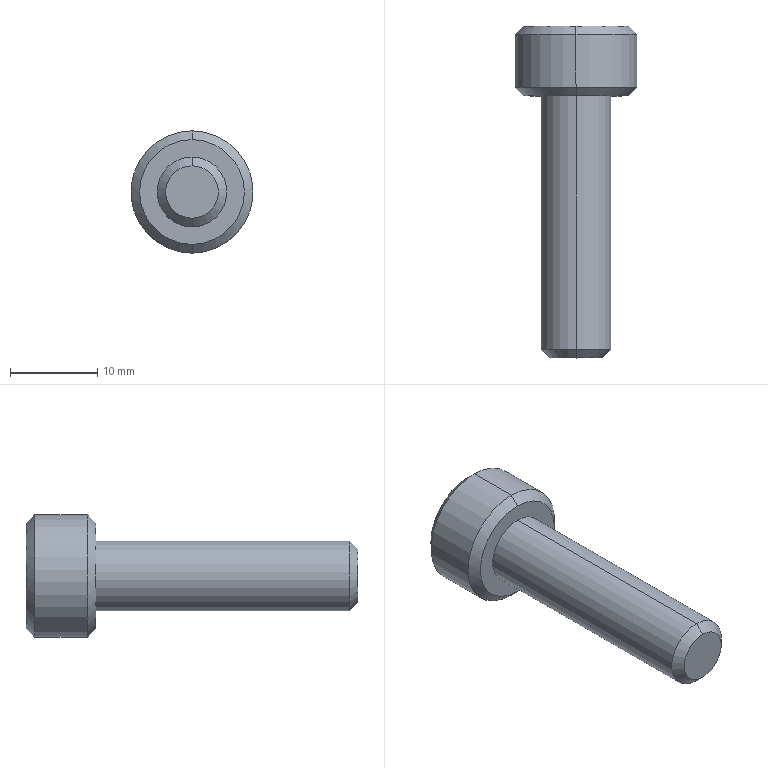Part | STEP file | Vibration plate 3-05_default | 1 solid | 20 faces | box 14 x 38 x 14 mm | volume 2499 mm3 | plane 10 | cone 6 | cylinder 4 | commonest cylinder face diameters 8 x2 14 x2
STEP:
#1=CARTESIAN_POINT('',(0.,0.,0.));
#2=DIRECTION('',(0.,0.,1.));
#3=DIRECTION('',(1.,0.,0.));
#4=AXIS2_PLACEMENT_3D('',#1,#2,#3);
#5=CARTESIAN_POINT('',(0.,1.,4.));
#6=VERTEX_POINT('',#5);
#7=CARTESIAN_POINT('',(0.,1.,-4.));
#8=VERTEX_POINT('',#7);
#9=CARTESIAN_POINT('',(0.,1.,0.));
#10=DIRECTION('',(0.,1.,0.));
#11=DIRECTION('',(0.,0.,1.));
#12=AXIS2_PLACEMENT_3D('',#9,#10,#11);
#13=CIRCLE('',#12,4.);
#14=CARTESIAN_POINT('',(0.,0.,0.));
#15=DIRECTION('',(0.,1.,0.));
#16=DIRECTION('',(0.,0.,1.));
#17=AXIS2_PLACEMENT_3D('',#14,#15,#16);
#18=CYLINDRICAL_SURFACE('',#17,4.);
#19=CARTESIAN_POINT('',(0.,1.));
#20=DIRECTION('',(1.,0.));
#21=VECTOR('',#20,1.);
#22=LINE('',#19,#21);
#23=(GEOMETRIC_REPRESENTATION_CONTEXT(2)PARAMETRIC_REPRESENTATION_CONTEXT()REPRESENTATION_CONTEXT('',''));
#24=DEFINITIONAL_REPRESENTATION('',(#22),#23);
#25=PCURVE('',#18,#24);
#26=CARTESIAN_POINT('',(0.,1.,0.));
#27=DIRECTION('',(0.,1.,0.));
#28=DIRECTION('',(0.,0.,1.));
#29=AXIS2_PLACEMENT_3D('',#26,#27,#28);
#30=CONICAL_SURFACE('',#29,4.,0.7854);
#31=CARTESIAN_POINT('',(0.,0.000008212));
#32=DIRECTION('',(1.,0.));
#33=VECTOR('',#32,1.);
#34=LINE('',#31,#33);
#35=(GEOMETRIC_REPRESENTATION_CONTEXT(2)PARAMETRIC_REPRESENTATION_CONTEXT()REPRESENTATION_CONTEXT('',''));
#36=DEFINITIONAL_REPRESENTATION('',(#34),#35);
#37=PCURVE('',#30,#36);
#38=SURFACE_CURVE('',#13,(#25,#37),.PCURVE_S1.);
#39=EDGE_CURVE('',#6,#8,#38,.T.);
#40=ORIENTED_EDGE('',*,*,#39,.T.);
#41=CARTESIAN_POINT('',(0.,30.,-4.));
#42=VERTEX_POINT('',#41);
#43=CARTESIAN_POINT('',(0.,0.,-4.));
#44=DIRECTION('',(0.,1.,0.));
#45=VECTOR('',#44,1.);
#46=LINE('',#43,#45);
#47=CARTESIAN_POINT('',(3.142,0.));
#48=DIRECTION('',(0.,1.));
#49=VECTOR('',#48,1.);
#50=LINE('',#47,#49);
#51=(GEOMETRIC_REPRESENTATION_CONTEXT(2)PARAMETRIC_REPRESENTATION_CONTEXT()REPRESENTATION_CONTEXT('',''));
#52=DEFINITIONAL_REPRESENTATION('',(#50),#51);
#53=PCURVE('',#18,#52);
#54=CARTESIAN_POINT('',(0.,0.,0.));
#55=DIRECTION('',(0.,1.,0.));
#56=DIRECTION('',(0.,0.,1.));
#57=AXIS2_PLACEMENT_3D('',#54,#55,#56);
#58=CYLINDRICAL_SURFACE('',#57,4.);
#59=CARTESIAN_POINT('',(3.142,0.));
#60=DIRECTION('',(0.,1.));
#61=VECTOR('',#60,1.);
#62=LINE('',#59,#61);
#63=(GEOMETRIC_REPRESENTATION_CONTEXT(2)PARAMETRIC_REPRESENTATION_CONTEXT()REPRESENTATION_CONTEXT('',''));
#64=DEFINITIONAL_REPRESENTATION('',(#62),#63);
#65=PCURVE('',#58,#64);
#66=SURFACE_CURVE('',#46,(#53,#65),.PCURVE_S1.);
#67=EDGE_CURVE('',#8,#42,#66,.T.);
#68=ORIENTED_EDGE('',*,*,#67,.T.);
#69=CARTESIAN_POINT('',(0.,30.,4.));
#70=VERTEX_POINT('',#69);
#71=CARTESIAN_POINT('',(0.,30.,0.));
#72=DIRECTION('',(0.,-1.,0.));
#73=DIRECTION('',(0.,0.,1.));
#74=AXIS2_PLACEMENT_3D('',#71,#72,#73);
#75=CIRCLE('',#74,4.);
#76=CARTESIAN_POINT('',(6.283,30.));
#77=DIRECTION('',(-1.,0.));
#78=VECTOR('',#77,1.);
#79=LINE('',#76,#78);
#80=(GEOMETRIC_REPRESENTATION_CONTEXT(2)PARAMETRIC_REPRESENTATION_CONTEXT()REPRESENTATION_CONTEXT('',''));
#81=DEFINITIONAL_REPRESENTATION('',(#79),#80);
#82=PCURVE('',#18,#81);
#83=CARTESIAN_POINT('',(0.,30.,0.));
#84=DIRECTION('',(0.,1.,0.));
#85=DIRECTION('',(0.,0.,1.));
#86=AXIS2_PLACEMENT_3D('',#83,#84,#85);
#87=PLANE('',#86);
#88=CARTESIAN_POINT('',(4.,0.));
#89=CARTESIAN_POINT('',(4.,-6.928));
#90=CARTESIAN_POINT('',(-2.,-3.464));
#91=CARTESIAN_POINT('',(-8.,0.));
#92=CARTESIAN_POINT('',(-2.,3.464));
#93=CARTESIAN_POINT('',(4.,6.928));
#94=CARTESIAN_POINT('',(4.,0.));
#95=(BOUNDED_CURVE()B_SPLINE_CURVE(2,(#88,#89,#90,#91,#92,#93,#94),.UNSPECIFIED.,.T.,.F.)B_SPLINE_CURVE_WITH_KNOTS((1,2,2,2,2,1),(-2.094,0.,2.094,4.189,6.283,8.378),.UNSPECIFIED.)CURVE()GEOMETRIC_REPRESENTATION_ITEM()RATIONAL_B_SPLINE_CURVE((1.,0.5,1.,0.5,1.,0.5,1.))REPRESENTATION_ITEM(''));
#96=(GEOMETRIC_REPRESENTATION_CONTEXT(2)PARAMETRIC_REPRESENTATION_CONTEXT()REPRESENTATION_CONTEXT('',''));
#97=DEFINITIONAL_REPRESENTATION('',(#95),#96);
#98=PCURVE('',#87,#97);
#99=SURFACE_CURVE('',#75,(#82,#98),.PCURVE_S1.);
#100=EDGE_CURVE('',#42,#70,#99,.T.);
#101=ORIENTED_EDGE('',*,*,#100,.T.);
#102=CARTESIAN_POINT('',(0.,0.,4.));
#103=DIRECTION('',(0.,1.,0.));
#104=VECTOR('',#103,1.);
#105=LINE('',#102,#104);
#106=CARTESIAN_POINT('',(0.,0.));
#107=DIRECTION('',(0.,1.));
#108=VECTOR('',#107,1.);
#109=LINE('',#106,#108);
#110=(GEOMETRIC_REPRESENTATION_CONTEXT(2)PARAMETRIC_REPRESENTATION_CONTEXT()REPRESENTATION_CONTEXT('',''));
#111=DEFINITIONAL_REPRESENTATION('',(#109),#110);
#112=PCURVE('',#18,#111);
#113=CARTESIAN_POINT('',(6.283,0.));
#114=DIRECTION('',(0.,1.));
#115=VECTOR('',#114,1.);
#116=LINE('',#113,#115);
#117=(GEOMETRIC_REPRESENTATION_CONTEXT(2)PARAMETRIC_REPRESENTATION_CONTEXT()REPRESENTATION_CONTEXT('',''));
#118=DEFINITIONAL_REPRESENTATION('',(#116),#117);
#119=PCURVE('',#58,#118);
#120=SURFACE_CURVE('',#105,(#112,#119),.PCURVE_S1.);
#121=EDGE_CURVE('',#6,#70,#120,.T.);
#122=ORIENTED_EDGE('',*,*,#121,.F.);
#123=EDGE_LOOP('',(#40,#68,#101,#122));
#124=FACE_BOUND('',#123,.T.);
#125=ADVANCED_FACE('',(#124),#18,.T.);
#126=CARTESIAN_POINT('',(0.,0.,3.));
#127=VERTEX_POINT('',#126);
#128=CARTESIAN_POINT('',(0.,0.,-3.));
#129=VERTEX_POINT('',#128);
#130=CARTESIAN_POINT('',(0.,0.,0.));
#131=DIRECTION('',(0.,1.,0.));
#132=DIRECTION('',(0.,0.,1.));
#133=AXIS2_PLACEMENT_3D('',#130,#131,#132);
#134=CIRCLE('',#133,3.);
#135=CARTESIAN_POINT('',(0.,-1.));
#136=DIRECTION('',(1.,0.));
#137=VECTOR('',#136,1.);
#138=LINE('',#135,#137);
#139=(GEOMETRIC_REPRESENTATION_CONTEXT(2)PARAMETRIC_REPRESENTATION_CONTEXT()REPRESENTATION_CONTEXT('',''));
#140=DEFINITIONAL_REPRESENTATION('',(#138),#139);
#141=PCURVE('',#30,#140);
#142=CARTESIAN_POINT('',(0.,0.,0.));
#143=DIRECTION('',(0.,1.,0.));
#144=DIRECTION('',(0.,0.,1.));
#145=AXIS2_PLACEMENT_3D('',#142,#143,#144);
#146=PLANE('',#145);
#147=CARTESIAN_POINT('',(0.,0.));
#148=DIRECTION('',(1.,0.));
#149=AXIS2_PLACEMENT_2D('',#147,#148);
#150=CIRCLE('',#149,3.);
#151=(GEOMETRIC_REPRESENTATION_CONTEXT(2)PARAMETRIC_REPRESENTATION_CONTEXT()REPRESENTATION_CONTEXT('',''));
#152=DEFINITIONAL_REPRESENTATION('',(#150),#151);
#153=PCURVE('',#146,#152);
#154=SURFACE_CURVE('',#134,(#141,#153),.PCURVE_S1.);
#155=EDGE_CURVE('',#127,#129,#154,.T.);
#156=ORIENTED_EDGE('',*,*,#155,.T.);
#157=CARTESIAN_POINT('',(0.,1.,-4.));
#158=DIRECTION('',(0.,0.7071,-0.7071));
#159=VECTOR('',#158,1.);
#160=LINE('',#157,#159);
#161=CARTESIAN_POINT('',(3.142,0.));
#162=DIRECTION('',(0.,1.));
#163=VECTOR('',#162,1.);
#164=LINE('',#161,#163);
#165=(GEOMETRIC_REPRESENTATION_CONTEXT(2)PARAMETRIC_REPRESENTATION_CONTEXT()REPRESENTATION_CONTEXT('',''));
#166=DEFINITIONAL_REPRESENTATION('',(#164),#165);
#167=PCURVE('',#30,#166);
#168=CARTESIAN_POINT('',(0.,1.,0.));
#169=DIRECTION('',(0.,1.,0.));
#170=DIRECTION('',(0.,0.,1.));
#171=AXIS2_PLACEMENT_3D('',#168,#169,#170);
#172=CONICAL_SURFACE('',#171,4.,0.7854);
#173=CARTESIAN_POINT('',(3.142,0.));
#174=DIRECTION('',(0.,1.));
#175=VECTOR('',#174,1.);
#176=LINE('',#173,#175);
#177=(GEOMETRIC_REPRESENTATION_CONTEXT(2)PARAMETRIC_REPRESENTATION_CONTEXT()REPRESENTATION_CONTEXT('',''));
#178=DEFINITIONAL_REPRESENTATION('',(#176),#177);
#179=PCURVE('',#172,#178);
#180=SURFACE_CURVE('',#160,(#167,#179),.PCURVE_S1.);
#181=EDGE_CURVE('',#129,#8,#180,.T.);
#182=ORIENTED_EDGE('',*,*,#181,.T.);
#183=ORIENTED_EDGE('',*,*,#39,.F.);
#184=CARTESIAN_POINT('',(0.,1.,4.));
#185=DIRECTION('',(0.,0.7071,0.7071));
#186=VECTOR('',#185,1.);
#187=LINE('',#184,#186);
#188=CARTESIAN_POINT('',(0.,0.));
#189=DIRECTION('',(0.,1.));
#190=VECTOR('',#189,1.);
#191=LINE('',#188,#190);
#192=(GEOMETRIC_REPRESENTATION_CONTEXT(2)PARAMETRIC_REPRESENTATION_CONTEXT()REPRESENTATION_CONTEXT('',''));
#193=DEFINITIONAL_REPRESENTATION('',(#191),#192);
#194=PCURVE('',#30,#193);
#195=CARTESIAN_POINT('',(6.283,0.));
#196=DIRECTION('',(0.,1.));
#197=VECTOR('',#196,1.);
#198=LINE('',#195,#197);
#199=(GEOMETRIC_REPRESENTATION_CONTEXT(2)PARAMETRIC_REPRESENTATION_CONTEXT()REPRESENTATION_CONTEXT('',''));
#200=DEFINITIONAL_REPRESENTATION('',(#198),#199);
#201=PCURVE('',#172,#200);
#202=SURFACE_CURVE('',#187,(#194,#201),.PCURVE_S1.);
#203=EDGE_CURVE('',#127,#6,#202,.T.);
#204=ORIENTED_EDGE('',*,*,#203,.F.);
#205=EDGE_LOOP('',(#156,#182,#183,#204));
#206=FACE_BOUND('',#205,.T.);
#207=ADVANCED_FACE('',(#206),#30,.T.);
#208=CARTESIAN_POINT('',(0.,30.,6.));
#209=VERTEX_POINT('',#208);
#210=CARTESIAN_POINT('',(0.,30.,-6.));
#211=VERTEX_POINT('',#210);
#212=CARTESIAN_POINT('',(0.,30.,0.));
#213=DIRECTION('',(0.,1.,0.));
#214=DIRECTION('',(0.,0.,1.));
#215=AXIS2_PLACEMENT_3D('',#212,#213,#214);
#216=CIRCLE('',#215,6.);
#217=CARTESIAN_POINT('',(0.,31.,0.));
#218=DIRECTION('',(0.,1.,0.));
#219=DIRECTION('',(0.,0.,1.));
#220=AXIS2_PLACEMENT_3D('',#217,#218,#219);
#221=CONICAL_SURFACE('',#220,7.,0.7854);
#222=CARTESIAN_POINT('',(0.,-1.));
#223=DIRECTION('',(1.,0.));
#224=VECTOR('',#223,1.);
#225=LINE('',#222,#224);
#226=(GEOMETRIC_REPRESENTATION_CONTEXT(2)PARAMETRIC_REPRESENTATION_CONTEXT()REPRESENTATION_CONTEXT('',''));
#227=DEFINITIONAL_REPRESENTATION('',(#225),#226);
#228=PCURVE('',#221,#227);
#229=CARTESIAN_POINT('',(0.,0.));
#230=DIRECTION('',(1.,0.));
#231=AXIS2_PLACEMENT_2D('',#229,#230);
#232=CIRCLE('',#231,6.);
#233=(GEOMETRIC_REPRESENTATION_CONTEXT(2)PARAMETRIC_REPRESENTATION_CONTEXT()REPRESENTATION_CONTEXT('',''));
#234=DEFINITIONAL_REPRESENTATION('',(#232),#233);
#235=PCURVE('',#87,#234);
#236=SURFACE_CURVE('',#216,(#228,#235),.PCURVE_S1.);
#237=EDGE_CURVE('',#209,#211,#236,.T.);
#238=ORIENTED_EDGE('',*,*,#237,.T.);
#239=CARTESIAN_POINT('',(0.,31.,-7.));
#240=VERTEX_POINT('',#239);
#241=CARTESIAN_POINT('',(0.,31.,-7.));
#242=DIRECTION('',(0.,0.7071,-0.7071));
#243=VECTOR('',#242,1.);
#244=LINE('',#241,#243);
#245=CARTESIAN_POINT('',(3.142,0.));
#246=DIRECTION('',(0.,1.));
#247=VECTOR('',#246,1.);
#248=LINE('',#245,#247);
#249=(GEOMETRIC_REPRESENTATION_CONTEXT(2)PARAMETRIC_REPRESENTATION_CONTEXT()REPRESENTATION_CONTEXT('',''));
#250=DEFINITIONAL_REPRESENTATION('',(#248),#249);
#251=PCURVE('',#221,#250);
#252=CARTESIAN_POINT('',(0.,31.,0.));
#253=DIRECTION('',(0.,1.,0.));
#254=DIRECTION('',(0.,0.,1.));
#255=AXIS2_PLACEMENT_3D('',#252,#253,#254);
#256=CONICAL_SURFACE('',#255,7.,0.7854);
#257=CARTESIAN_POINT('',(3.142,0.));
#258=DIRECTION('',(0.,1.));
#259=VECTOR('',#258,1.);
#260=LINE('',#257,#259);
#261=(GEOMETRIC_REPRESENTATION_CONTEXT(2)PARAMETRIC_REPRESENTATION_CONTEXT()REPRESENTATION_CONTEXT('',''));
#262=DEFINITIONAL_REPRESENTATION('',(#260),#261);
#263=PCURVE('',#256,#262);
#264=SURFACE_CURVE('',#244,(#251,#263),.PCURVE_S1.);
#265=EDGE_CURVE('',#211,#240,#264,.T.);
#266=ORIENTED_EDGE('',*,*,#265,.T.);
#267=CARTESIAN_POINT('',(0.,31.,7.));
#268=VERTEX_POINT('',#267);
#269=CARTESIAN_POINT('',(0.,31.,0.));
#270=DIRECTION('',(0.,-1.,0.));
#271=DIRECTION('',(0.,0.,-1.));
#272=AXIS2_PLACEMENT_3D('',#269,#270,#271);
#273=CIRCLE('',#272,7.);
#274=CARTESIAN_POINT('',(3.142,0.));
#275=DIRECTION('',(-1.,0.));
#276=VECTOR('',#275,1.);
#277=LINE('',#274,#276);
#278=(GEOMETRIC_REPRESENTATION_CONTEXT(2)PARAMETRIC_REPRESENTATION_CONTEXT()REPRESENTATION_CONTEXT('',''));
#279=DEFINITIONAL_REPRESENTATION('',(#277),#278);
#280=PCURVE('',#221,#279);
#281=CARTESIAN_POINT('',(0.,30.,0.));
#282=DIRECTION('',(0.,1.,0.));
#283=DIRECTION('',(0.,0.,1.));
#284=AXIS2_PLACEMENT_3D('',#281,#282,#283);
#285=CYLINDRICAL_SURFACE('',#284,7.);
#286=CARTESIAN_POINT('',(3.142,1.));
#287=DIRECTION('',(-1.,0.));
#288=VECTOR('',#287,1.);
#289=LINE('',#286,#288);
#290=(GEOMETRIC_REPRESENTATION_CONTEXT(2)PARAMETRIC_REPRESENTATION_CONTEXT()REPRESENTATION_CONTEXT('',''));
#291=DEFINITIONAL_REPRESENTATION('',(#289),#290);
#292=PCURVE('',#285,#291);
#293=SURFACE_CURVE('',#273,(#280,#292),.PCURVE_S1.);
#294=EDGE_CURVE('',#240,#268,#293,.T.);
#295=ORIENTED_EDGE('',*,*,#294,.T.);
#296=CARTESIAN_POINT('',(0.,31.,7.));
#297=DIRECTION('',(0.,0.7071,0.7071));
#298=VECTOR('',#297,1.);
#299=LINE('',#296,#298);
#300=CARTESIAN_POINT('',(0.,0.));
#301=DIRECTION('',(0.,1.));
#302=VECTOR('',#301,1.);
#303=LINE('',#300,#302);
#304=(GEOMETRIC_REPRESENTATION_CONTEXT(2)PARAMETRIC_REPRESENTATION_CONTEXT()REPRESENTATION_CONTEXT('',''));
#305=DEFINITIONAL_REPRESENTATION('',(#303),#304);
#306=PCURVE('',#221,#305);
#307=CARTESIAN_POINT('',(6.283,0.));
#308=DIRECTION('',(0.,1.));
#309=VECTOR('',#308,1.);
#310=LINE('',#307,#309);
#311=(GEOMETRIC_REPRESENTATION_CONTEXT(2)PARAMETRIC_REPRESENTATION_CONTEXT()REPRESENTATION_CONTEXT('',''));
#312=DEFINITIONAL_REPRESENTATION('',(#310),#311);
#313=PCURVE('',#256,#312);
#314=SURFACE_CURVE('',#299,(#306,#313),.PCURVE_S1.);
#315=EDGE_CURVE('',#209,#268,#314,.T.);
#316=ORIENTED_EDGE('',*,*,#315,.F.);
#317=EDGE_LOOP('',(#238,#266,#295,#316));
#318=FACE_BOUND('',#317,.T.);
#319=ADVANCED_FACE('',(#318),#221,.T.);
#320=ORIENTED_EDGE('',*,*,#294,.F.);
#321=CARTESIAN_POINT('',(0.,37.,-7.));
#322=VERTEX_POINT('',#321);
#323=CARTESIAN_POINT('',(0.,30.,-7.));
#324=DIRECTION('',(0.,1.,0.));
#325=VECTOR('',#324,1.);
#326=LINE('',#323,#325);
#327=CARTESIAN_POINT('',(3.142,0.));
#328=DIRECTION('',(0.,1.));
#329=VECTOR('',#328,1.);
#330=LINE('',#327,#329);
#331=(GEOMETRIC_REPRESENTATION_CONTEXT(2)PARAMETRIC_REPRESENTATION_CONTEXT()REPRESENTATION_CONTEXT('',''));
#332=DEFINITIONAL_REPRESENTATION('',(#330),#331);
#333=PCURVE('',#285,#332);
#334=CARTESIAN_POINT('',(0.,30.,0.));
#335=DIRECTION('',(0.,1.,0.));
#336=DIRECTION('',(0.,0.,1.));
#337=AXIS2_PLACEMENT_3D('',#334,#335,#336);
#338=CYLINDRICAL_SURFACE('',#337,7.);
#339=CARTESIAN_POINT('',(3.142,0.));
#340=DIRECTION('',(0.,1.));
#341=VECTOR('',#340,1.);
#342=LINE('',#339,#341);
#343=(GEOMETRIC_REPRESENTATION_CONTEXT(2)PARAMETRIC_REPRESENTATION_CONTEXT()REPRESENTATION_CONTEXT('',''));
#344=DEFINITIONAL_REPRESENTATION('',(#342),#343);
#345=PCURVE('',#338,#344);
#346=SURFACE_CURVE('',#326,(#333,#345),.PCURVE_S1.);
#347=EDGE_CURVE('',#240,#322,#346,.T.);
#348=ORIENTED_EDGE('',*,*,#347,.T.);
#349=CARTESIAN_POINT('',(0.,37.,7.));
#350=VERTEX_POINT('',#349);
#351=CARTESIAN_POINT('',(0.,37.,0.));
#352=DIRECTION('',(0.,-1.,0.));
#353=DIRECTION('',(0.,0.,1.));
#354=AXIS2_PLACEMENT_3D('',#351,#352,#353);
#355=CIRCLE('',#354,7.);
#356=CARTESIAN_POINT('',(6.283,7.));
#357=DIRECTION('',(-1.,0.));
#358=VECTOR('',#357,1.);
#359=LINE('',#356,#358);
#360=(GEOMETRIC_REPRESENTATION_CONTEXT(2)PARAMETRIC_REPRESENTATION_CONTEXT()REPRESENTATION_CONTEXT('',''));
#361=DEFINITIONAL_REPRESENTATION('',(#359),#360);
#362=PCURVE('',#285,#361);
#363=CARTESIAN_POINT('',(0.,37.,0.));
#364=DIRECTION('',(0.,-1.,0.));
#365=DIRECTION('',(0.,0.,-1.));
#366=AXIS2_PLACEMENT_3D('',#363,#364,#365);
#367=CONICAL_SURFACE('',#366,7.,0.7854);
#368=CARTESIAN_POINT('',(-3.142,0.000000446));
#369=DIRECTION('',(1.,0.));
#370=VECTOR('',#369,1.);
#371=LINE('',#368,#370);
#372=(GEOMETRIC_REPRESENTATION_CONTEXT(2)PARAMETRIC_REPRESENTATION_CONTEXT()REPRESENTATION_CONTEXT('',''));
#373=DEFINITIONAL_REPRESENTATION('',(#371),#372);
#374=PCURVE('',#367,#373);
#375=SURFACE_CURVE('',#355,(#362,#374),.PCURVE_S1.);
#376=EDGE_CURVE('',#322,#350,#375,.T.);
#377=ORIENTED_EDGE('',*,*,#376,.T.);
#378=CARTESIAN_POINT('',(0.,30.,7.));
#379=DIRECTION('',(0.,1.,0.));
#380=VECTOR('',#379,1.);
#381=LINE('',#378,#380);
#382=CARTESIAN_POINT('',(0.,0.));
#383=DIRECTION('',(0.,1.));
#384=VECTOR('',#383,1.);
#385=LINE('',#382,#384);
#386=(GEOMETRIC_REPRESENTATION_CONTEXT(2)PARAMETRIC_REPRESENTATION_CONTEXT()REPRESENTATION_CONTEXT('',''));
#387=DEFINITIONAL_REPRESENTATION('',(#385),#386);
#388=PCURVE('',#285,#387);
#389=CARTESIAN_POINT('',(6.283,0.));
#390=DIRECTION('',(0.,1.));
#391=VECTOR('',#390,1.);
#392=LINE('',#389,#391);
#393=(GEOMETRIC_REPRESENTATION_CONTEXT(2)PARAMETRIC_REPRESENTATION_CONTEXT()REPRESENTATION_CONTEXT('',''));
#394=DEFINITIONAL_REPRESENTATION('',(#392),#393);
#395=PCURVE('',#338,#394);
#396=SURFACE_CURVE('',#381,(#388,#395),.PCURVE_S1.);
#397=EDGE_CURVE('',#268,#350,#396,.T.);
#398=ORIENTED_EDGE('',*,*,#397,.F.);
#399=EDGE_LOOP('',(#320,#348,#377,#398));
#400=FACE_BOUND('',#399,.T.);
#401=ADVANCED_FACE('',(#400),#285,.T.);
#402=CARTESIAN_POINT('',(0.,38.,-6.));
#403=VERTEX_POINT('',#402);
#404=CARTESIAN_POINT('',(0.,38.,6.));
#405=VERTEX_POINT('',#404);
#406=CARTESIAN_POINT('',(0.,38.,0.));
#407=DIRECTION('',(0.,-1.,0.));
#408=DIRECTION('',(0.,0.,-1.));
#409=AXIS2_PLACEMENT_3D('',#406,#407,#408);
#410=CIRCLE('',#409,6.);
#411=CARTESIAN_POINT('',(0.,-1.));
#412=DIRECTION('',(1.,0.));
#413=VECTOR('',#412,1.);
#414=LINE('',#411,#413);
#415=(GEOMETRIC_REPRESENTATION_CONTEXT(2)PARAMETRIC_REPRESENTATION_CONTEXT()REPRESENTATION_CONTEXT('',''));
#416=DEFINITIONAL_REPRESENTATION('',(#414),#415);
#417=PCURVE('',#367,#416);
#418=CARTESIAN_POINT('',(0.,38.,0.));
#419=DIRECTION('',(0.,1.,0.));
#420=DIRECTION('',(0.,0.,1.));
#421=AXIS2_PLACEMENT_3D('',#418,#419,#420);
#422=PLANE('',#421);
#423=CARTESIAN_POINT('',(-6.,0.));
#424=CARTESIAN_POINT('',(-6.,10.392));
#425=CARTESIAN_POINT('',(3.,5.196));
#426=CARTESIAN_POINT('',(12.,0.));
#427=CARTESIAN_POINT('',(3.,-5.196));
#428=CARTESIAN_POINT('',(-6.,-10.392));
#429=CARTESIAN_POINT('',(-6.,0.));
#430=(BOUNDED_CURVE()B_SPLINE_CURVE(2,(#423,#424,#425,#426,#427,#428,#429),.UNSPECIFIED.,.T.,.F.)B_SPLINE_CURVE_WITH_KNOTS((1,2,2,2,2,1),(-2.094,0.,2.094,4.189,6.283,8.378),.UNSPECIFIED.)CURVE()GEOMETRIC_REPRESENTATION_ITEM()RATIONAL_B_SPLINE_CURVE((1.,0.5,1.,0.5,1.,0.5,1.))REPRESENTATION_ITEM(''));
#431=(GEOMETRIC_REPRESENTATION_CONTEXT(2)PARAMETRIC_REPRESENTATION_CONTEXT()REPRESENTATION_CONTEXT('',''));
#432=DEFINITIONAL_REPRESENTATION('',(#430),#431);
#433=PCURVE('',#422,#432);
#434=SURFACE_CURVE('',#410,(#417,#433),.PCURVE_S1.);
#435=EDGE_CURVE('',#403,#405,#434,.T.);
#436=ORIENTED_EDGE('',*,*,#435,.T.);
#437=CARTESIAN_POINT('',(0.,37.,7.));
#438=DIRECTION('',(0.,-0.7071,0.7071));
#439=VECTOR('',#438,1.);
#440=LINE('',#437,#439);
#441=CARTESIAN_POINT('',(3.142,0.));
#442=DIRECTION('',(0.,1.));
#443=VECTOR('',#442,1.);
#444=LINE('',#441,#443);
#445=(GEOMETRIC_REPRESENTATION_CONTEXT(2)PARAMETRIC_REPRESENTATION_CONTEXT()REPRESENTATION_CONTEXT('',''));
#446=DEFINITIONAL_REPRESENTATION('',(#444),#445);
#447=PCURVE('',#367,#446);
#448=CARTESIAN_POINT('',(0.,37.,0.));
#449=DIRECTION('',(0.,-1.,0.));
#450=DIRECTION('',(0.,0.,-1.));
#451=AXIS2_PLACEMENT_3D('',#448,#449,#450);
#452=CONICAL_SURFACE('',#451,7.,0.7854);
#453=CARTESIAN_POINT('',(3.142,0.));
#454=DIRECTION('',(0.,1.));
#455=VECTOR('',#454,1.);
#456=LINE('',#453,#455);
#457=(GEOMETRIC_REPRESENTATION_CONTEXT(2)PARAMETRIC_REPRESENTATION_CONTEXT()REPRESENTATION_CONTEXT('',''));
#458=DEFINITIONAL_REPRESENTATION('',(#456),#457);
#459=PCURVE('',#452,#458);
#460=SURFACE_CURVE('',#440,(#447,#459),.PCURVE_S1.);
#461=EDGE_CURVE('',#405,#350,#460,.T.);
#462=ORIENTED_EDGE('',*,*,#461,.T.);
#463=ORIENTED_EDGE('',*,*,#376,.F.);
#464=CARTESIAN_POINT('',(0.,37.,-7.));
#465=DIRECTION('',(0.,-0.7071,-0.7071));
#466=VECTOR('',#465,1.);
#467=LINE('',#464,#466);
#468=CARTESIAN_POINT('',(0.,0.));
#469=DIRECTION('',(0.,1.));
#470=VECTOR('',#469,1.);
#471=LINE('',#468,#470);
#472=(GEOMETRIC_REPRESENTATION_CONTEXT(2)PARAMETRIC_REPRESENTATION_CONTEXT()REPRESENTATION_CONTEXT('',''));
#473=DEFINITIONAL_REPRESENTATION('',(#471),#472);
#474=PCURVE('',#367,#473);
#475=CARTESIAN_POINT('',(6.283,0.));
#476=DIRECTION('',(0.,1.));
#477=VECTOR('',#476,1.);
#478=LINE('',#475,#477);
#479=(GEOMETRIC_REPRESENTATION_CONTEXT(2)PARAMETRIC_REPRESENTATION_CONTEXT()REPRESENTATION_CONTEXT('',''));
#480=DEFINITIONAL_REPRESENTATION('',(#478),#479);
#481=PCURVE('',#452,#480);
#482=SURFACE_CURVE('',#467,(#474,#481),.PCURVE_S1.);
#483=EDGE_CURVE('',#403,#322,#482,.T.);
#484=ORIENTED_EDGE('',*,*,#483,.F.);
#485=EDGE_LOOP('',(#436,#462,#463,#484));
#486=FACE_BOUND('',#485,.T.);
#487=ADVANCED_FACE('',(#486),#367,.T.);
#488=ORIENTED_EDGE('',*,*,#67,.F.);
#489=CARTESIAN_POINT('',(0.,1.,0.));
#490=DIRECTION('',(0.,1.,0.));
#491=DIRECTION('',(0.,0.,1.));
#492=AXIS2_PLACEMENT_3D('',#489,#490,#491);
#493=CIRCLE('',#492,4.);
#494=CARTESIAN_POINT('',(0.,1.));
#495=DIRECTION('',(1.,0.));
#496=VECTOR('',#495,1.);
#497=LINE('',#494,#496);
#498=(GEOMETRIC_REPRESENTATION_CONTEXT(2)PARAMETRIC_REPRESENTATION_CONTEXT()REPRESENTATION_CONTEXT('',''));
#499=DEFINITIONAL_REPRESENTATION('',(#497),#498);
#500=PCURVE('',#58,#499);
#501=CARTESIAN_POINT('',(0.,0.000008212));
#502=DIRECTION('',(1.,0.));
#503=VECTOR('',#502,1.);
#504=LINE('',#501,#503);
#505=(GEOMETRIC_REPRESENTATION_CONTEXT(2)PARAMETRIC_REPRESENTATION_CONTEXT()REPRESENTATION_CONTEXT('',''));
#506=DEFINITIONAL_REPRESENTATION('',(#504),#505);
#507=PCURVE('',#172,#506);
#508=SURFACE_CURVE('',#493,(#500,#507),.PCURVE_S1.);
#509=EDGE_CURVE('',#8,#6,#508,.T.);
#510=ORIENTED_EDGE('',*,*,#509,.T.);
#511=ORIENTED_EDGE('',*,*,#121,.T.);
#512=CARTESIAN_POINT('',(0.,30.,0.));
#513=DIRECTION('',(0.,-1.,0.));
#514=DIRECTION('',(0.,0.,1.));
#515=AXIS2_PLACEMENT_3D('',#512,#513,#514);
#516=CIRCLE('',#515,4.);
#517=CARTESIAN_POINT('',(6.283,30.));
#518=DIRECTION('',(-1.,0.));
#519=VECTOR('',#518,1.);
#520=LINE('',#517,#519);
#521=(GEOMETRIC_REPRESENTATION_CONTEXT(2)PARAMETRIC_REPRESENTATION_CONTEXT()REPRESENTATION_CONTEXT('',''));
#522=DEFINITIONAL_REPRESENTATION('',(#520),#521);
#523=PCURVE('',#58,#522);
#524=CARTESIAN_POINT('',(4.,0.));
#525=CARTESIAN_POINT('',(4.,-6.928));
#526=CARTESIAN_POINT('',(-2.,-3.464));
#527=CARTESIAN_POINT('',(-8.,0.));
#528=CARTESIAN_POINT('',(-2.,3.464));
#529=CARTESIAN_POINT('',(4.,6.928));
#530=CARTESIAN_POINT('',(4.,0.));
#531=(BOUNDED_CURVE()B_SPLINE_CURVE(2,(#524,#525,#526,#527,#528,#529,#530),.UNSPECIFIED.,.T.,.F.)B_SPLINE_CURVE_WITH_KNOTS((1,2,2,2,2,1),(-2.094,0.,2.094,4.189,6.283,8.378),.UNSPECIFIED.)CURVE()GEOMETRIC_REPRESENTATION_ITEM()RATIONAL_B_SPLINE_CURVE((1.,0.5,1.,0.5,1.,0.5,1.))REPRESENTATION_ITEM(''));
#532=(GEOMETRIC_REPRESENTATION_CONTEXT(2)PARAMETRIC_REPRESENTATION_CONTEXT()REPRESENTATION_CONTEXT('',''));
#533=DEFINITIONAL_REPRESENTATION('',(#531),#532);
#534=PCURVE('',#87,#533);
#535=SURFACE_CURVE('',#516,(#523,#534),.PCURVE_S1.);
#536=EDGE_CURVE('',#70,#42,#535,.T.);
#537=ORIENTED_EDGE('',*,*,#536,.T.);
#538=EDGE_LOOP('',(#488,#510,#511,#537));
#539=FACE_BOUND('',#538,.T.);
#540=ADVANCED_FACE('',(#539),#58,.T.);
#541=ORIENTED_EDGE('',*,*,#181,.F.);
#542=CARTESIAN_POINT('',(0.,0.,0.));
#543=DIRECTION('',(0.,1.,0.));
#544=DIRECTION('',(0.,0.,1.));
#545=AXIS2_PLACEMENT_3D('',#542,#543,#544);
#546=CIRCLE('',#545,3.);
#547=CARTESIAN_POINT('',(0.,-1.));
#548=DIRECTION('',(1.,0.));
#549=VECTOR('',#548,1.);
#550=LINE('',#547,#549);
#551=(GEOMETRIC_REPRESENTATION_CONTEXT(2)PARAMETRIC_REPRESENTATION_CONTEXT()REPRESENTATION_CONTEXT('',''));
#552=DEFINITIONAL_REPRESENTATION('',(#550),#551);
#553=PCURVE('',#172,#552);
#554=CARTESIAN_POINT('',(0.,0.));
#555=DIRECTION('',(1.,0.));
#556=AXIS2_PLACEMENT_2D('',#554,#555);
#557=CIRCLE('',#556,3.);
#558=(GEOMETRIC_REPRESENTATION_CONTEXT(2)PARAMETRIC_REPRESENTATION_CONTEXT()REPRESENTATION_CONTEXT('',''));
#559=DEFINITIONAL_REPRESENTATION('',(#557),#558);
#560=PCURVE('',#146,#559);
#561=SURFACE_CURVE('',#546,(#553,#560),.PCURVE_S1.);
#562=EDGE_CURVE('',#129,#127,#561,.T.);
#563=ORIENTED_EDGE('',*,*,#562,.T.);
#564=ORIENTED_EDGE('',*,*,#203,.T.);
#565=ORIENTED_EDGE('',*,*,#509,.F.);
#566=EDGE_LOOP('',(#541,#563,#564,#565));
#567=FACE_BOUND('',#566,.T.);
#568=ADVANCED_FACE('',(#567),#172,.T.);
#569=ORIENTED_EDGE('',*,*,#536,.F.);
#570=ORIENTED_EDGE('',*,*,#100,.F.);
#571=EDGE_LOOP('',(#569,#570));
#572=FACE_BOUND('',#571,.T.);
#573=CARTESIAN_POINT('',(0.,30.,0.));
#574=DIRECTION('',(0.,1.,0.));
#575=DIRECTION('',(0.,0.,1.));
#576=AXIS2_PLACEMENT_3D('',#573,#574,#575);
#577=CIRCLE('',#576,6.);
#578=CARTESIAN_POINT('',(0.,0.));
#579=DIRECTION('',(1.,0.));
#580=AXIS2_PLACEMENT_2D('',#578,#579);
#581=CIRCLE('',#580,6.);
#582=(GEOMETRIC_REPRESENTATION_CONTEXT(2)PARAMETRIC_REPRESENTATION_CONTEXT()REPRESENTATION_CONTEXT('',''));
#583=DEFINITIONAL_REPRESENTATION('',(#581),#582);
#584=PCURVE('',#87,#583);
#585=CARTESIAN_POINT('',(0.,-1.));
#586=DIRECTION('',(1.,0.));
#587=VECTOR('',#586,1.);
#588=LINE('',#585,#587);
#589=(GEOMETRIC_REPRESENTATION_CONTEXT(2)PARAMETRIC_REPRESENTATION_CONTEXT()REPRESENTATION_CONTEXT('',''));
#590=DEFINITIONAL_REPRESENTATION('',(#588),#589);
#591=PCURVE('',#256,#590);
#592=SURFACE_CURVE('',#577,(#584,#591),.PCURVE_S1.);
#593=EDGE_CURVE('',#211,#209,#592,.T.);
#594=ORIENTED_EDGE('',*,*,#593,.T.);
#595=ORIENTED_EDGE('',*,*,#237,.T.);
#596=EDGE_LOOP('',(#594,#595));
#597=FACE_BOUND('',#596,.F.);
#598=ADVANCED_FACE('',(#572,#597),#87,.F.);
#599=ORIENTED_EDGE('',*,*,#155,.F.);
#600=ORIENTED_EDGE('',*,*,#562,.F.);
#601=EDGE_LOOP('',(#599,#600));
#602=FACE_BOUND('',#601,.T.);
#603=ADVANCED_FACE('',(#602),#146,.F.);
#604=ORIENTED_EDGE('',*,*,#265,.F.);
#605=ORIENTED_EDGE('',*,*,#593,.T.);
#606=ORIENTED_EDGE('',*,*,#315,.T.);
#607=CARTESIAN_POINT('',(0.,31.,0.));
#608=DIRECTION('',(0.,-1.,0.));
#609=DIRECTION('',(0.,0.,-1.));
#610=AXIS2_PLACEMENT_3D('',#607,#608,#609);
#611=CIRCLE('',#610,7.);
#612=CARTESIAN_POINT('',(9.425,0.));
#613=DIRECTION('',(-1.,0.));
#614=VECTOR('',#613,1.);
#615=LINE('',#612,#614);
#616=(GEOMETRIC_REPRESENTATION_CONTEXT(2)PARAMETRIC_REPRESENTATION_CONTEXT()REPRESENTATION_CONTEXT('',''));
#617=DEFINITIONAL_REPRESENTATION('',(#615),#616);
#618=PCURVE('',#256,#617);
#619=CARTESIAN_POINT('',(9.425,1.));
#620=DIRECTION('',(-1.,0.));
#621=VECTOR('',#620,1.);
#622=LINE('',#619,#621);
#623=(GEOMETRIC_REPRESENTATION_CONTEXT(2)PARAMETRIC_REPRESENTATION_CONTEXT()REPRESENTATION_CONTEXT('',''));
#624=DEFINITIONAL_REPRESENTATION('',(#622),#623);
#625=PCURVE('',#338,#624);
#626=SURFACE_CURVE('',#611,(#618,#625),.PCURVE_S1.);
#627=EDGE_CURVE('',#268,#240,#626,.T.);
#628=ORIENTED_EDGE('',*,*,#627,.T.);
#629=EDGE_LOOP('',(#604,#605,#606,#628));
#630=FACE_BOUND('',#629,.T.);
#631=ADVANCED_FACE('',(#630),#256,.T.);
#632=ORIENTED_EDGE('',*,*,#347,.F.);
#633=ORIENTED_EDGE('',*,*,#627,.F.);
#634=ORIENTED_EDGE('',*,*,#397,.T.);
#635=CARTESIAN_POINT('',(0.,37.,0.));
#636=DIRECTION('',(0.,-1.,0.));
#637=DIRECTION('',(0.,0.,1.));
#638=AXIS2_PLACEMENT_3D('',#635,#636,#637);
#639=CIRCLE('',#638,7.);
#640=CARTESIAN_POINT('',(6.283,7.));
#641=DIRECTION('',(-1.,0.));
#642=VECTOR('',#641,1.);
#643=LINE('',#640,#642);
#644=(GEOMETRIC_REPRESENTATION_CONTEXT(2)PARAMETRIC_REPRESENTATION_CONTEXT()REPRESENTATION_CONTEXT('',''));
#645=DEFINITIONAL_REPRESENTATION('',(#643),#644);
#646=PCURVE('',#338,#645);
#647=CARTESIAN_POINT('',(3.142,0.000000446));
#648=DIRECTION('',(1.,0.));
#649=VECTOR('',#648,1.);
#650=LINE('',#647,#649);
#651=(GEOMETRIC_REPRESENTATION_CONTEXT(2)PARAMETRIC_REPRESENTATION_CONTEXT()REPRESENTATION_CONTEXT('',''));
#652=DEFINITIONAL_REPRESENTATION('',(#650),#651);
#653=PCURVE('',#452,#652);
#654=SURFACE_CURVE('',#639,(#646,#653),.PCURVE_S1.);
#655=EDGE_CURVE('',#350,#322,#654,.T.);
#656=ORIENTED_EDGE('',*,*,#655,.T.);
#657=EDGE_LOOP('',(#632,#633,#634,#656));
#658=FACE_BOUND('',#657,.T.);
#659=ADVANCED_FACE('',(#658),#338,.T.);
#660=ORIENTED_EDGE('',*,*,#461,.F.);
#661=CARTESIAN_POINT('',(0.,38.,0.));
#662=DIRECTION('',(0.,-1.,0.));
#663=DIRECTION('',(0.,0.,-1.));
#664=AXIS2_PLACEMENT_3D('',#661,#662,#663);
#665=CIRCLE('',#664,6.);
#666=CARTESIAN_POINT('',(0.,-1.));
#667=DIRECTION('',(1.,0.));
#668=VECTOR('',#667,1.);
#669=LINE('',#666,#668);
#670=(GEOMETRIC_REPRESENTATION_CONTEXT(2)PARAMETRIC_REPRESENTATION_CONTEXT()REPRESENTATION_CONTEXT('',''));
#671=DEFINITIONAL_REPRESENTATION('',(#669),#670);
#672=PCURVE('',#452,#671);
#673=CARTESIAN_POINT('',(-6.,0.));
#674=CARTESIAN_POINT('',(-6.,10.392));
#675=CARTESIAN_POINT('',(3.,5.196));
#676=CARTESIAN_POINT('',(12.,0.));
#677=CARTESIAN_POINT('',(3.,-5.196));
#678=CARTESIAN_POINT('',(-6.,-10.392));
#679=CARTESIAN_POINT('',(-6.,0.));
#680=(BOUNDED_CURVE()B_SPLINE_CURVE(2,(#673,#674,#675,#676,#677,#678,#679),.UNSPECIFIED.,.T.,.F.)B_SPLINE_CURVE_WITH_KNOTS((1,2,2,2,2,1),(-2.094,0.,2.094,4.189,6.283,8.378),.UNSPECIFIED.)CURVE()GEOMETRIC_REPRESENTATION_ITEM()RATIONAL_B_SPLINE_CURVE((1.,0.5,1.,0.5,1.,0.5,1.))REPRESENTATION_ITEM(''));
#681=(GEOMETRIC_REPRESENTATION_CONTEXT(2)PARAMETRIC_REPRESENTATION_CONTEXT()REPRESENTATION_CONTEXT('',''));
#682=DEFINITIONAL_REPRESENTATION('',(#680),#681);
#683=PCURVE('',#422,#682);
#684=SURFACE_CURVE('',#665,(#672,#683),.PCURVE_S1.);
#685=EDGE_CURVE('',#405,#403,#684,.T.);
#686=ORIENTED_EDGE('',*,*,#685,.T.);
#687=ORIENTED_EDGE('',*,*,#483,.T.);
#688=ORIENTED_EDGE('',*,*,#655,.F.);
#689=EDGE_LOOP('',(#660,#686,#687,#688));
#690=FACE_BOUND('',#689,.T.);
#691=ADVANCED_FACE('',(#690),#452,.T.);
#692=CARTESIAN_POINT('',(1.7,38.,-3.));
#693=VERTEX_POINT('',#692);
#694=CARTESIAN_POINT('',(3.432,38.,0.));
#695=VERTEX_POINT('',#694);
#696=CARTESIAN_POINT('',(1.7,38.,-3.));
#697=DIRECTION('',(0.5,0.,0.866));
#698=VECTOR('',#697,1.);
#699=LINE('',#696,#698);
#700=CARTESIAN_POINT('',(-3.,1.7));
#701=DIRECTION('',(0.866,0.5));
#702=VECTOR('',#701,1.);
#703=LINE('',#700,#702);
#704=(GEOMETRIC_REPRESENTATION_CONTEXT(2)PARAMETRIC_REPRESENTATION_CONTEXT()REPRESENTATION_CONTEXT('',''));
#705=DEFINITIONAL_REPRESENTATION('',(#703),#704);
#706=PCURVE('',#422,#705);
#707=CARTESIAN_POINT('',(3.432,38.,0.));
#708=DIRECTION('',(0.866,0.,-0.5));
#709=DIRECTION('',(-0.5,0.,-0.866));
#710=AXIS2_PLACEMENT_3D('',#707,#708,#709);
#711=PLANE('',#710);
#712=CARTESIAN_POINT('',(3.464,0.));
#713=DIRECTION('',(-1.,0.));
#714=VECTOR('',#713,1.);
#715=LINE('',#712,#714);
#716=(GEOMETRIC_REPRESENTATION_CONTEXT(2)PARAMETRIC_REPRESENTATION_CONTEXT()REPRESENTATION_CONTEXT('',''));
#717=DEFINITIONAL_REPRESENTATION('',(#715),#716);
#718=PCURVE('',#711,#717);
#719=SURFACE_CURVE('',#699,(#706,#718),.PCURVE_S1.);
#720=EDGE_CURVE('',#693,#695,#719,.T.);
#721=ORIENTED_EDGE('',*,*,#720,.T.);
#722=CARTESIAN_POINT('',(1.7,38.,3.));
#723=VERTEX_POINT('',#722);
#724=CARTESIAN_POINT('',(3.432,38.,0.));
#725=DIRECTION('',(-0.5,0.,0.866));
#726=VECTOR('',#725,1.);
#727=LINE('',#724,#726);
#728=CARTESIAN_POINT('',(0.,3.432));
#729=DIRECTION('',(0.866,-0.5));
#730=VECTOR('',#729,1.);
#731=LINE('',#728,#730);
#732=(GEOMETRIC_REPRESENTATION_CONTEXT(2)PARAMETRIC_REPRESENTATION_CONTEXT()REPRESENTATION_CONTEXT('',''));
#733=DEFINITIONAL_REPRESENTATION('',(#731),#732);
#734=PCURVE('',#422,#733);
#735=CARTESIAN_POINT('',(1.7,38.,3.));
#736=DIRECTION('',(0.866,0.,0.5));
#737=DIRECTION('',(0.5,0.,-0.866));
#738=AXIS2_PLACEMENT_3D('',#735,#736,#737);
#739=PLANE('',#738);
#740=CARTESIAN_POINT('',(3.464,0.));
#741=DIRECTION('',(-1.,0.));
#742=VECTOR('',#741,1.);
#743=LINE('',#740,#742);
#744=(GEOMETRIC_REPRESENTATION_CONTEXT(2)PARAMETRIC_REPRESENTATION_CONTEXT()REPRESENTATION_CONTEXT('',''));
#745=DEFINITIONAL_REPRESENTATION('',(#743),#744);
#746=PCURVE('',#739,#745);
#747=SURFACE_CURVE('',#727,(#734,#746),.PCURVE_S1.);
#748=EDGE_CURVE('',#695,#723,#747,.T.);
#749=ORIENTED_EDGE('',*,*,#748,.T.);
#750=CARTESIAN_POINT('',(-1.764,38.,3.));
#751=VERTEX_POINT('',#750);
#752=CARTESIAN_POINT('',(0.,38.,3.));
#753=DIRECTION('',(-1.,0.,0.));
#754=VECTOR('',#753,1.);
#755=LINE('',#752,#754);
#756=CARTESIAN_POINT('',(3.,0.));
#757=DIRECTION('',(0.,-1.));
#758=VECTOR('',#757,1.);
#759=LINE('',#756,#758);
#760=(GEOMETRIC_REPRESENTATION_CONTEXT(2)PARAMETRIC_REPRESENTATION_CONTEXT()REPRESENTATION_CONTEXT('',''));
#761=DEFINITIONAL_REPRESENTATION('',(#759),#760);
#762=PCURVE('',#422,#761);
#763=CARTESIAN_POINT('',(-1.764,38.,3.));
#764=DIRECTION('',(0.,0.,1.));
#765=DIRECTION('',(1.,0.,0.));
#766=AXIS2_PLACEMENT_3D('',#763,#764,#765);
#767=PLANE('',#766);
#768=CARTESIAN_POINT('',(1.764,0.));
#769=DIRECTION('',(-1.,0.));
#770=VECTOR('',#769,1.);
#771=LINE('',#768,#770);
#772=(GEOMETRIC_REPRESENTATION_CONTEXT(2)PARAMETRIC_REPRESENTATION_CONTEXT()REPRESENTATION_CONTEXT('',''));
#773=DEFINITIONAL_REPRESENTATION('',(#771),#772);
#774=PCURVE('',#767,#773);
#775=SURFACE_CURVE('',#755,(#762,#774),.PCURVE_S1.);
#776=EDGE_CURVE('',#723,#751,#775,.T.);
#777=ORIENTED_EDGE('',*,*,#776,.T.);
#778=CARTESIAN_POINT('',(-3.496,38.,0.));
#779=VERTEX_POINT('',#778);
#780=CARTESIAN_POINT('',(-1.764,38.,3.));
#781=DIRECTION('',(-0.5,0.,-0.866));
#782=VECTOR('',#781,1.);
#783=LINE('',#780,#782);
#784=CARTESIAN_POINT('',(3.,-1.764));
#785=DIRECTION('',(-0.866,-0.5));
#786=VECTOR('',#785,1.);
#787=LINE('',#784,#786);
#788=(GEOMETRIC_REPRESENTATION_CONTEXT(2)PARAMETRIC_REPRESENTATION_CONTEXT()REPRESENTATION_CONTEXT('',''));
#789=DEFINITIONAL_REPRESENTATION('',(#787),#788);
#790=PCURVE('',#422,#789);
#791=CARTESIAN_POINT('',(-3.496,38.,0.));
#792=DIRECTION('',(-0.866,0.,0.5));
#793=DIRECTION('',(0.5,0.,0.866));
#794=AXIS2_PLACEMENT_3D('',#791,#792,#793);
#795=PLANE('',#794);
#796=CARTESIAN_POINT('',(3.464,0.));
#797=DIRECTION('',(-1.,0.));
#798=VECTOR('',#797,1.);
#799=LINE('',#796,#798);
#800=(GEOMETRIC_REPRESENTATION_CONTEXT(2)PARAMETRIC_REPRESENTATION_CONTEXT()REPRESENTATION_CONTEXT('',''));
#801=DEFINITIONAL_REPRESENTATION('',(#799),#800);
#802=PCURVE('',#795,#801);
#803=SURFACE_CURVE('',#783,(#790,#802),.PCURVE_S1.);
#804=EDGE_CURVE('',#751,#779,#803,.T.);
#805=ORIENTED_EDGE('',*,*,#804,.T.);
#806=CARTESIAN_POINT('',(-1.764,38.,-3.));
#807=VERTEX_POINT('',#806);
#808=CARTESIAN_POINT('',(-3.496,38.,0.));
#809=DIRECTION('',(0.5,0.,-0.866));
#810=VECTOR('',#809,1.);
#811=LINE('',#808,#810);
#812=CARTESIAN_POINT('',(0.,-3.496));
#813=DIRECTION('',(-0.866,0.5));
#814=VECTOR('',#813,1.);
#815=LINE('',#812,#814);
#816=(GEOMETRIC_REPRESENTATION_CONTEXT(2)PARAMETRIC_REPRESENTATION_CONTEXT()REPRESENTATION_CONTEXT('',''));
#817=DEFINITIONAL_REPRESENTATION('',(#815),#816);
#818=PCURVE('',#422,#817);
#819=CARTESIAN_POINT('',(-1.764,38.,-3.));
#820=DIRECTION('',(-0.866,0.,-0.5));
#821=DIRECTION('',(-0.5,0.,0.866));
#822=AXIS2_PLACEMENT_3D('',#819,#820,#821);
#823=PLANE('',#822);
#824=CARTESIAN_POINT('',(3.464,0.));
#825=DIRECTION('',(-1.,0.));
#826=VECTOR('',#825,1.);
#827=LINE('',#824,#826);
#828=(GEOMETRIC_REPRESENTATION_CONTEXT(2)PARAMETRIC_REPRESENTATION_CONTEXT()REPRESENTATION_CONTEXT('',''));
#829=DEFINITIONAL_REPRESENTATION('',(#827),#828);
#830=PCURVE('',#823,#829);
#831=SURFACE_CURVE('',#811,(#818,#830),.PCURVE_S1.);
#832=EDGE_CURVE('',#779,#807,#831,.T.);
#833=ORIENTED_EDGE('',*,*,#832,.T.);
#834=CARTESIAN_POINT('',(0.,38.,-3.));
#835=DIRECTION('',(1.,0.,0.));
#836=VECTOR('',#835,1.);
#837=LINE('',#834,#836);
#838=CARTESIAN_POINT('',(-3.,0.));
#839=DIRECTION('',(0.,1.));
#840=VECTOR('',#839,1.);
#841=LINE('',#838,#840);
#842=(GEOMETRIC_REPRESENTATION_CONTEXT(2)PARAMETRIC_REPRESENTATION_CONTEXT()REPRESENTATION_CONTEXT('',''));
#843=DEFINITIONAL_REPRESENTATION('',(#841),#842);
#844=PCURVE('',#422,#843);
#845=CARTESIAN_POINT('',(1.7,38.,-3.));
#846=DIRECTION('',(0.,0.,-1.));
#847=DIRECTION('',(-1.,0.,0.));
#848=AXIS2_PLACEMENT_3D('',#845,#846,#847);
#849=PLANE('',#848);
#850=CARTESIAN_POINT('',(1.7,0.));
#851=DIRECTION('',(-1.,0.));
#852=VECTOR('',#851,1.);
#853=LINE('',#850,#852);
#854=(GEOMETRIC_REPRESENTATION_CONTEXT(2)PARAMETRIC_REPRESENTATION_CONTEXT()REPRESENTATION_CONTEXT('',''));
#855=DEFINITIONAL_REPRESENTATION('',(#853),#854);
#856=PCURVE('',#849,#855);
#857=SURFACE_CURVE('',#837,(#844,#856),.PCURVE_S1.);
#858=EDGE_CURVE('',#807,#693,#857,.T.);
#859=ORIENTED_EDGE('',*,*,#858,.T.);
#860=EDGE_LOOP('',(#721,#749,#777,#805,#833,#859));
#861=FACE_BOUND('',#860,.T.);
#862=ORIENTED_EDGE('',*,*,#435,.F.);
#863=ORIENTED_EDGE('',*,*,#685,.F.);
#864=EDGE_LOOP('',(#862,#863));
#865=FACE_BOUND('',#864,.T.);
#866=ADVANCED_FACE('',(#861,#865),#422,.T.);
#867=CARTESIAN_POINT('',(1.7,32.,3.));
#868=VERTEX_POINT('',#867);
#869=CARTESIAN_POINT('',(3.432,32.,0.));
#870=VERTEX_POINT('',#869);
#871=CARTESIAN_POINT('',(1.7,32.,3.));
#872=DIRECTION('',(0.5,0.,-0.866));
#873=VECTOR('',#872,1.);
#874=LINE('',#871,#873);
#875=CARTESIAN_POINT('',(0.,-6.));
#876=DIRECTION('',(1.,0.));
#877=VECTOR('',#876,1.);
#878=LINE('',#875,#877);
#879=(GEOMETRIC_REPRESENTATION_CONTEXT(2)PARAMETRIC_REPRESENTATION_CONTEXT()REPRESENTATION_CONTEXT('',''));
#880=DEFINITIONAL_REPRESENTATION('',(#878),#879);
#881=PCURVE('',#739,#880);
#882=CARTESIAN_POINT('',(0.,32.,0.));
#883=DIRECTION('',(0.,1.,0.));
#884=DIRECTION('',(0.,0.,1.));
#885=AXIS2_PLACEMENT_3D('',#882,#883,#884);
#886=PLANE('',#885);
#887=CARTESIAN_POINT('',(3.,1.7));
#888=DIRECTION('',(-0.866,0.5));
#889=VECTOR('',#888,1.);
#890=LINE('',#887,#889);
#891=(GEOMETRIC_REPRESENTATION_CONTEXT(2)PARAMETRIC_REPRESENTATION_CONTEXT()REPRESENTATION_CONTEXT('',''));
#892=DEFINITIONAL_REPRESENTATION('',(#890),#891);
#893=PCURVE('',#886,#892);
#894=SURFACE_CURVE('',#874,(#881,#893),.PCURVE_S1.);
#895=EDGE_CURVE('',#868,#870,#894,.T.);
#896=ORIENTED_EDGE('',*,*,#895,.F.);
#897=CARTESIAN_POINT('',(1.7,38.,3.));
#898=DIRECTION('',(0.,-1.,0.));
#899=VECTOR('',#898,1.);
#900=LINE('',#897,#899);
#901=CARTESIAN_POINT('',(0.,0.));
#902=DIRECTION('',(0.,-1.));
#903=VECTOR('',#902,1.);
#904=LINE('',#901,#903);
#905=(GEOMETRIC_REPRESENTATION_CONTEXT(2)PARAMETRIC_REPRESENTATION_CONTEXT()REPRESENTATION_CONTEXT('',''));
#906=DEFINITIONAL_REPRESENTATION('',(#904),#905);
#907=PCURVE('',#739,#906);
#908=CARTESIAN_POINT('',(3.464,0.));
#909=DIRECTION('',(0.,-1.));
#910=VECTOR('',#909,1.);
#911=LINE('',#908,#910);
#912=(GEOMETRIC_REPRESENTATION_CONTEXT(2)PARAMETRIC_REPRESENTATION_CONTEXT()REPRESENTATION_CONTEXT('',''));
#913=DEFINITIONAL_REPRESENTATION('',(#911),#912);
#914=PCURVE('',#767,#913);
#915=SURFACE_CURVE('',#900,(#907,#914),.PCURVE_S1.);
#916=EDGE_CURVE('',#723,#868,#915,.T.);
#917=ORIENTED_EDGE('',*,*,#916,.F.);
#918=ORIENTED_EDGE('',*,*,#748,.F.);
#919=CARTESIAN_POINT('',(3.432,38.,0.));
#920=DIRECTION('',(0.,1.,0.));
#921=VECTOR('',#920,1.);
#922=LINE('',#919,#921);
#923=CARTESIAN_POINT('',(3.464,0.));
#924=DIRECTION('',(0.,1.));
#925=VECTOR('',#924,1.);
#926=LINE('',#923,#925);
#927=(GEOMETRIC_REPRESENTATION_CONTEXT(2)PARAMETRIC_REPRESENTATION_CONTEXT()REPRESENTATION_CONTEXT('',''));
#928=DEFINITIONAL_REPRESENTATION('',(#926),#927);
#929=PCURVE('',#739,#928);
#930=CARTESIAN_POINT('',(0.,0.));
#931=DIRECTION('',(0.,1.));
#932=VECTOR('',#931,1.);
#933=LINE('',#930,#932);
#934=(GEOMETRIC_REPRESENTATION_CONTEXT(2)PARAMETRIC_REPRESENTATION_CONTEXT()REPRESENTATION_CONTEXT('',''));
#935=DEFINITIONAL_REPRESENTATION('',(#933),#934);
#936=PCURVE('',#711,#935);
#937=SURFACE_CURVE('',#922,(#929,#936),.PCURVE_S1.);
#938=EDGE_CURVE('',#870,#695,#937,.T.);
#939=ORIENTED_EDGE('',*,*,#938,.F.);
#940=EDGE_LOOP('',(#896,#917,#918,#939));
#941=FACE_BOUND('',#940,.T.);
#942=ADVANCED_FACE('',(#941),#739,.F.);
#943=CARTESIAN_POINT('',(1.7,32.,-3.));
#944=VERTEX_POINT('',#943);
#945=CARTESIAN_POINT('',(3.432,32.,0.));
#946=DIRECTION('',(-0.5,0.,-0.866));
#947=VECTOR('',#946,1.);
#948=LINE('',#945,#947);
#949=CARTESIAN_POINT('',(0.,-6.));
#950=DIRECTION('',(1.,0.));
#951=VECTOR('',#950,1.);
#952=LINE('',#949,#951);
#953=(GEOMETRIC_REPRESENTATION_CONTEXT(2)PARAMETRIC_REPRESENTATION_CONTEXT()REPRESENTATION_CONTEXT('',''));
#954=DEFINITIONAL_REPRESENTATION('',(#952),#953);
#955=PCURVE('',#711,#954);
#956=CARTESIAN_POINT('',(0.,3.432));
#957=DIRECTION('',(-0.866,-0.5));
#958=VECTOR('',#957,1.);
#959=LINE('',#956,#958);
#960=(GEOMETRIC_REPRESENTATION_CONTEXT(2)PARAMETRIC_REPRESENTATION_CONTEXT()REPRESENTATION_CONTEXT('',''));
#961=DEFINITIONAL_REPRESENTATION('',(#959),#960);
#962=PCURVE('',#886,#961);
#963=SURFACE_CURVE('',#948,(#955,#962),.PCURVE_S1.);
#964=EDGE_CURVE('',#870,#944,#963,.T.);
#965=ORIENTED_EDGE('',*,*,#964,.F.);
#966=ORIENTED_EDGE('',*,*,#938,.T.);
#967=ORIENTED_EDGE('',*,*,#720,.F.);
#968=CARTESIAN_POINT('',(1.7,38.,-3.));
#969=DIRECTION('',(0.,1.,0.));
#970=VECTOR('',#969,1.);
#971=LINE('',#968,#970);
#972=CARTESIAN_POINT('',(3.464,0.));
#973=DIRECTION('',(0.,1.));
#974=VECTOR('',#973,1.);
#975=LINE('',#972,#974);
#976=(GEOMETRIC_REPRESENTATION_CONTEXT(2)PARAMETRIC_REPRESENTATION_CONTEXT()REPRESENTATION_CONTEXT('',''));
#977=DEFINITIONAL_REPRESENTATION('',(#975),#976);
#978=PCURVE('',#711,#977);
#979=CARTESIAN_POINT('',(0.,0.));
#980=DIRECTION('',(0.,1.));
#981=VECTOR('',#980,1.);
#982=LINE('',#979,#981);
#983=(GEOMETRIC_REPRESENTATION_CONTEXT(2)PARAMETRIC_REPRESENTATION_CONTEXT()REPRESENTATION_CONTEXT('',''));
#984=DEFINITIONAL_REPRESENTATION('',(#982),#983);
#985=PCURVE('',#849,#984);
#986=SURFACE_CURVE('',#971,(#978,#985),.PCURVE_S1.);
#987=EDGE_CURVE('',#944,#693,#986,.T.);
#988=ORIENTED_EDGE('',*,*,#987,.F.);
#989=EDGE_LOOP('',(#965,#966,#967,#988));
#990=FACE_BOUND('',#989,.T.);
#991=ADVANCED_FACE('',(#990),#711,.F.);
#992=CARTESIAN_POINT('',(-1.764,32.,-3.));
#993=VERTEX_POINT('',#992);
#994=CARTESIAN_POINT('',(1.7,32.,-3.));
#995=DIRECTION('',(-1.,0.,0.));
#996=VECTOR('',#995,1.);
#997=LINE('',#994,#996);
#998=CARTESIAN_POINT('',(0.,-6.));
#999=DIRECTION('',(1.,0.));
#1000=VECTOR('',#999,1.);
#1001=LINE('',#998,#1000);
#1002=(GEOMETRIC_REPRESENTATION_CONTEXT(2)PARAMETRIC_REPRESENTATION_CONTEXT()REPRESENTATION_CONTEXT('',''));
#1003=DEFINITIONAL_REPRESENTATION('',(#1001),#1002);
#1004=PCURVE('',#849,#1003);
#1005=CARTESIAN_POINT('',(-3.,1.7));
#1006=DIRECTION('',(0.,-1.));
#1007=VECTOR('',#1006,1.);
#1008=LINE('',#1005,#1007);
#1009=(GEOMETRIC_REPRESENTATION_CONTEXT(2)PARAMETRIC_REPRESENTATION_CONTEXT()REPRESENTATION_CONTEXT('',''));
#1010=DEFINITIONAL_REPRESENTATION('',(#1008),#1009);
#1011=PCURVE('',#886,#1010);
#1012=SURFACE_CURVE('',#997,(#1004,#1011),.PCURVE_S1.);
#1013=EDGE_CURVE('',#944,#993,#1012,.T.);
#1014=ORIENTED_EDGE('',*,*,#1013,.F.);
#1015=ORIENTED_EDGE('',*,*,#987,.T.);
#1016=ORIENTED_EDGE('',*,*,#858,.F.);
#1017=CARTESIAN_POINT('',(-1.764,38.,-3.));
#1018=DIRECTION('',(0.,1.,0.));
#1019=VECTOR('',#1018,1.);
#1020=LINE('',#1017,#1019);
#1021=CARTESIAN_POINT('',(3.464,0.));
#1022=DIRECTION('',(0.,1.));
#1023=VECTOR('',#1022,1.);
#1024=LINE('',#1021,#1023);
#1025=(GEOMETRIC_REPRESENTATION_CONTEXT(2)PARAMETRIC_REPRESENTATION_CONTEXT()REPRESENTATION_CONTEXT('',''));
#1026=DEFINITIONAL_REPRESENTATION('',(#1024),#1025);
#1027=PCURVE('',#849,#1026);
#1028=CARTESIAN_POINT('',(0.,0.));
#1029=DIRECTION('',(0.,1.));
#1030=VECTOR('',#1029,1.);
#1031=LINE('',#1028,#1030);
#1032=(GEOMETRIC_REPRESENTATION_CONTEXT(2)PARAMETRIC_REPRESENTATION_CONTEXT()REPRESENTATION_CONTEXT('',''));
#1033=DEFINITIONAL_REPRESENTATION('',(#1031),#1032);
#1034=PCURVE('',#823,#1033);
#1035=SURFACE_CURVE('',#1020,(#1027,#1034),.PCURVE_S1.);
#1036=EDGE_CURVE('',#993,#807,#1035,.T.);
#1037=ORIENTED_EDGE('',*,*,#1036,.F.);
#1038=EDGE_LOOP('',(#1014,#1015,#1016,#1037));
#1039=FACE_BOUND('',#1038,.T.);
#1040=ADVANCED_FACE('',(#1039),#849,.F.);
#1041=CARTESIAN_POINT('',(-3.496,32.,0.));
#1042=VERTEX_POINT('',#1041);
#1043=CARTESIAN_POINT('',(-1.764,32.,-3.));
#1044=DIRECTION('',(-0.5,0.,0.866));
#1045=VECTOR('',#1044,1.);
#1046=LINE('',#1043,#1045);
#1047=CARTESIAN_POINT('',(0.,-6.));
#1048=DIRECTION('',(1.,0.));
#1049=VECTOR('',#1048,1.);
#1050=LINE('',#1047,#1049);
#1051=(GEOMETRIC_REPRESENTATION_CONTEXT(2)PARAMETRIC_REPRESENTATION_CONTEXT()REPRESENTATION_CONTEXT('',''));
#1052=DEFINITIONAL_REPRESENTATION('',(#1050),#1051);
#1053=PCURVE('',#823,#1052);
#1054=CARTESIAN_POINT('',(-3.,-1.764));
#1055=DIRECTION('',(0.866,-0.5));
#1056=VECTOR('',#1055,1.);
#1057=LINE('',#1054,#1056);
#1058=(GEOMETRIC_REPRESENTATION_CONTEXT(2)PARAMETRIC_REPRESENTATION_CONTEXT()REPRESENTATION_CONTEXT('',''));
#1059=DEFINITIONAL_REPRESENTATION('',(#1057),#1058);
#1060=PCURVE('',#886,#1059);
#1061=SURFACE_CURVE('',#1046,(#1053,#1060),.PCURVE_S1.);
#1062=EDGE_CURVE('',#993,#1042,#1061,.T.);
#1063=ORIENTED_EDGE('',*,*,#1062,.F.);
#1064=ORIENTED_EDGE('',*,*,#1036,.T.);
#1065=ORIENTED_EDGE('',*,*,#832,.F.);
#1066=CARTESIAN_POINT('',(-3.496,38.,0.));
#1067=DIRECTION('',(0.,1.,0.));
#1068=VECTOR('',#1067,1.);
#1069=LINE('',#1066,#1068);
#1070=CARTESIAN_POINT('',(3.464,0.));
#1071=DIRECTION('',(0.,1.));
#1072=VECTOR('',#1071,1.);
#1073=LINE('',#1070,#1072);
#1074=(GEOMETRIC_REPRESENTATION_CONTEXT(2)PARAMETRIC_REPRESENTATION_CONTEXT()REPRESENTATION_CONTEXT('',''));
#1075=DEFINITIONAL_REPRESENTATION('',(#1073),#1074);
#1076=PCURVE('',#823,#1075);
#1077=CARTESIAN_POINT('',(0.,0.));
#1078=DIRECTION('',(0.,1.));
#1079=VECTOR('',#1078,1.);
#1080=LINE('',#1077,#1079);
#1081=(GEOMETRIC_REPRESENTATION_CONTEXT(2)PARAMETRIC_REPRESENTATION_CONTEXT()REPRESENTATION_CONTEXT('',''));
#1082=DEFINITIONAL_REPRESENTATION('',(#1080),#1081);
#1083=PCURVE('',#795,#1082);
#1084=SURFACE_CURVE('',#1069,(#1076,#1083),.PCURVE_S1.);
#1085=EDGE_CURVE('',#1042,#779,#1084,.T.);
#1086=ORIENTED_EDGE('',*,*,#1085,.F.);
#1087=EDGE_LOOP('',(#1063,#1064,#1065,#1086));
#1088=FACE_BOUND('',#1087,.T.);
#1089=ADVANCED_FACE('',(#1088),#823,.F.);
#1090=CARTESIAN_POINT('',(-1.764,32.,3.));
#1091=VERTEX_POINT('',#1090);
#1092=CARTESIAN_POINT('',(-3.496,32.,0.));
#1093=DIRECTION('',(0.5,0.,0.866));
#1094=VECTOR('',#1093,1.);
#1095=LINE('',#1092,#1094);
#1096=CARTESIAN_POINT('',(0.,-6.));
#1097=DIRECTION('',(1.,0.));
#1098=VECTOR('',#1097,1.);
#1099=LINE('',#1096,#1098);
#1100=(GEOMETRIC_REPRESENTATION_CONTEXT(2)PARAMETRIC_REPRESENTATION_CONTEXT()REPRESENTATION_CONTEXT('',''));
#1101=DEFINITIONAL_REPRESENTATION('',(#1099),#1100);
#1102=PCURVE('',#795,#1101);
#1103=CARTESIAN_POINT('',(0.,-3.496));
#1104=DIRECTION('',(0.866,0.5));
#1105=VECTOR('',#1104,1.);
#1106=LINE('',#1103,#1105);
#1107=(GEOMETRIC_REPRESENTATION_CONTEXT(2)PARAMETRIC_REPRESENTATION_CONTEXT()REPRESENTATION_CONTEXT('',''));
#1108=DEFINITIONAL_REPRESENTATION('',(#1106),#1107);
#1109=PCURVE('',#886,#1108);
#1110=SURFACE_CURVE('',#1095,(#1102,#1109),.PCURVE_S1.);
#1111=EDGE_CURVE('',#1042,#1091,#1110,.T.);
#1112=ORIENTED_EDGE('',*,*,#1111,.F.);
#1113=ORIENTED_EDGE('',*,*,#1085,.T.);
#1114=ORIENTED_EDGE('',*,*,#804,.F.);
#1115=CARTESIAN_POINT('',(-1.764,38.,3.));
#1116=DIRECTION('',(0.,1.,0.));
#1117=VECTOR('',#1116,1.);
#1118=LINE('',#1115,#1117);
#1119=CARTESIAN_POINT('',(3.464,0.));
#1120=DIRECTION('',(0.,1.));
#1121=VECTOR('',#1120,1.);
#1122=LINE('',#1119,#1121);
#1123=(GEOMETRIC_REPRESENTATION_CONTEXT(2)PARAMETRIC_REPRESENTATION_CONTEXT()REPRESENTATION_CONTEXT('',''));
#1124=DEFINITIONAL_REPRESENTATION('',(#1122),#1123);
#1125=PCURVE('',#795,#1124);
#1126=CARTESIAN_POINT('',(0.,0.));
#1127=DIRECTION('',(0.,1.));
#1128=VECTOR('',#1127,1.);
#1129=LINE('',#1126,#1128);
#1130=(GEOMETRIC_REPRESENTATION_CONTEXT(2)PARAMETRIC_REPRESENTATION_CONTEXT()REPRESENTATION_CONTEXT('',''));
#1131=DEFINITIONAL_REPRESENTATION('',(#1129),#1130);
#1132=PCURVE('',#767,#1131);
#1133=SURFACE_CURVE('',#1118,(#1125,#1132),.PCURVE_S1.);
#1134=EDGE_CURVE('',#1091,#751,#1133,.T.);
#1135=ORIENTED_EDGE('',*,*,#1134,.F.);
#1136=EDGE_LOOP('',(#1112,#1113,#1114,#1135));
#1137=FACE_BOUND('',#1136,.T.);
#1138=ADVANCED_FACE('',(#1137),#795,.F.);
#1139=CARTESIAN_POINT('',(-1.764,32.,3.));
#1140=DIRECTION('',(1.,0.,0.));
#1141=VECTOR('',#1140,1.);
#1142=LINE('',#1139,#1141);
#1143=CARTESIAN_POINT('',(0.,-6.));
#1144=DIRECTION('',(1.,0.));
#1145=VECTOR('',#1144,1.);
#1146=LINE('',#1143,#1145);
#1147=(GEOMETRIC_REPRESENTATION_CONTEXT(2)PARAMETRIC_REPRESENTATION_CONTEXT()REPRESENTATION_CONTEXT('',''));
#1148=DEFINITIONAL_REPRESENTATION('',(#1146),#1147);
#1149=PCURVE('',#767,#1148);
#1150=CARTESIAN_POINT('',(3.,-1.764));
#1151=DIRECTION('',(0.,1.));
#1152=VECTOR('',#1151,1.);
#1153=LINE('',#1150,#1152);
#1154=(GEOMETRIC_REPRESENTATION_CONTEXT(2)PARAMETRIC_REPRESENTATION_CONTEXT()REPRESENTATION_CONTEXT('',''));
#1155=DEFINITIONAL_REPRESENTATION('',(#1153),#1154);
#1156=PCURVE('',#886,#1155);
#1157=SURFACE_CURVE('',#1142,(#1149,#1156),.PCURVE_S1.);
#1158=EDGE_CURVE('',#1091,#868,#1157,.T.);
#1159=ORIENTED_EDGE('',*,*,#1158,.F.);
#1160=ORIENTED_EDGE('',*,*,#1134,.T.);
#1161=ORIENTED_EDGE('',*,*,#776,.F.);
#1162=ORIENTED_EDGE('',*,*,#916,.T.);
#1163=EDGE_LOOP('',(#1159,#1160,#1161,#1162));
#1164=FACE_BOUND('',#1163,.T.);
#1165=ADVANCED_FACE('',(#1164),#767,.F.);
#1166=ORIENTED_EDGE('',*,*,#1158,.T.);
#1167=ORIENTED_EDGE('',*,*,#895,.T.);
#1168=ORIENTED_EDGE('',*,*,#964,.T.);
#1169=ORIENTED_EDGE('',*,*,#1013,.T.);
#1170=ORIENTED_EDGE('',*,*,#1062,.T.);
#1171=ORIENTED_EDGE('',*,*,#1111,.T.);
#1172=EDGE_LOOP('',(#1166,#1167,#1168,#1169,#1170,#1171));
#1173=FACE_BOUND('',#1172,.T.);
#1174=ADVANCED_FACE('',(#1173),#886,.T.);
#1175=CLOSED_SHELL('',(#125,#207,#319,#401,#487,#540,#568,#598,#603,#631,#659,#691,#866,#942,#991,#1040,#1089,#1138,#1165,#1174));
#1176=MANIFOLD_SOLID_BREP('',#1175);
#1177=(LENGTH_UNIT()NAMED_UNIT(*)SI_UNIT(.MILLI.,.METRE.));
#1178=UNCERTAINTY_MEASURE_WITH_UNIT(LENGTH_MEASURE(0.0000002),#1177,'','');
#1179=(NAMED_UNIT(*)PLANE_ANGLE_UNIT()SI_UNIT($,.RADIAN.));
#1180=(NAMED_UNIT(*)SI_UNIT($,.STERADIAN.)SOLID_ANGLE_UNIT());
#1181=(GEOMETRIC_REPRESENTATION_CONTEXT(3)GLOBAL_UNCERTAINTY_ASSIGNED_CONTEXT((#1178))GLOBAL_UNIT_ASSIGNED_CONTEXT((#1177,#1179,#1180))REPRESENTATION_CONTEXT('',''));
#1182=ADVANCED_BREP_SHAPE_REPRESENTATION('',(#4,#1176),#1181);